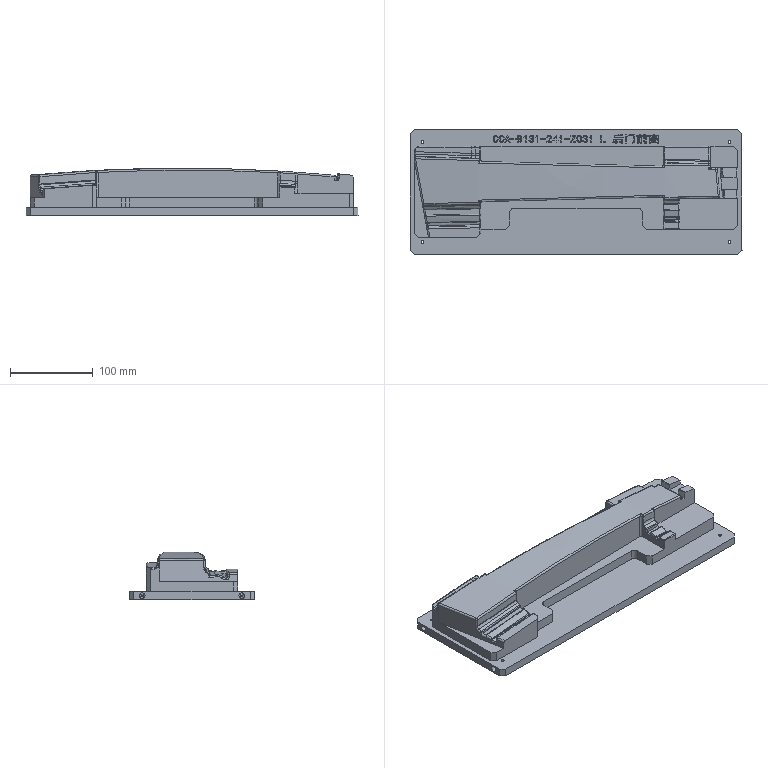Part | 2 solids | 672 faces | box 400 x 150 x 57.494 mm | volume 1730222 mm3 | spline 339 | plane 243 | cylinder 63 | sphere 22 | cone 4 | torus 1 | commonest cylinder face diameters 2 x25 4 x24 3.4 x8 6.8 x4 10 x2